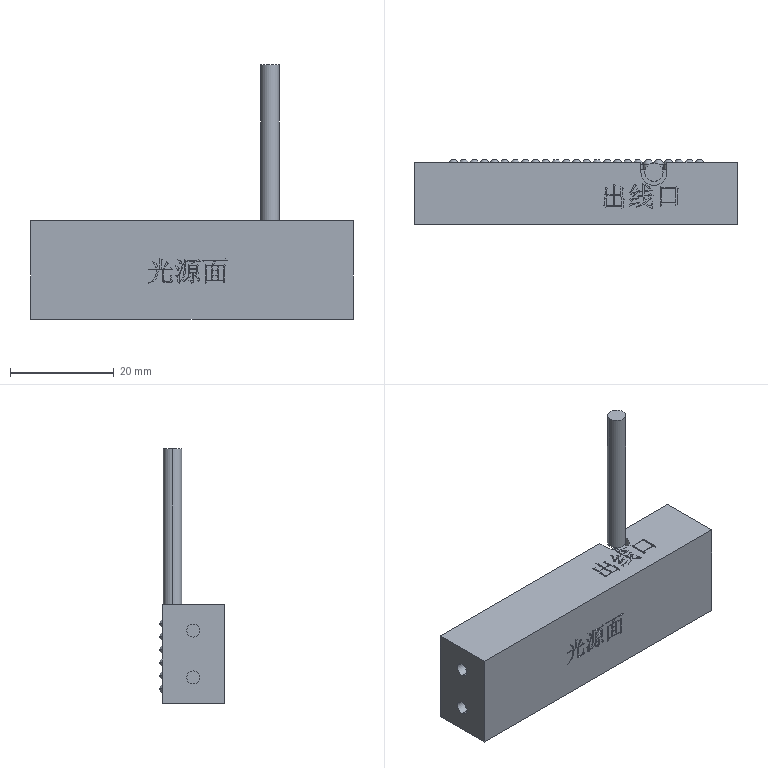Part | NX | features BREP 2 | 2 solids | 878 faces | box 62 x 12.5 x 49 mm | volume 13782 mm3 | cylinder 308 | sphere 300 | plane 227 | spline 43 | commonest cylinder face diameters 1.8 x275 2.5 x8 2.527 x2 3.5 x2 5 x1 7.456 x1